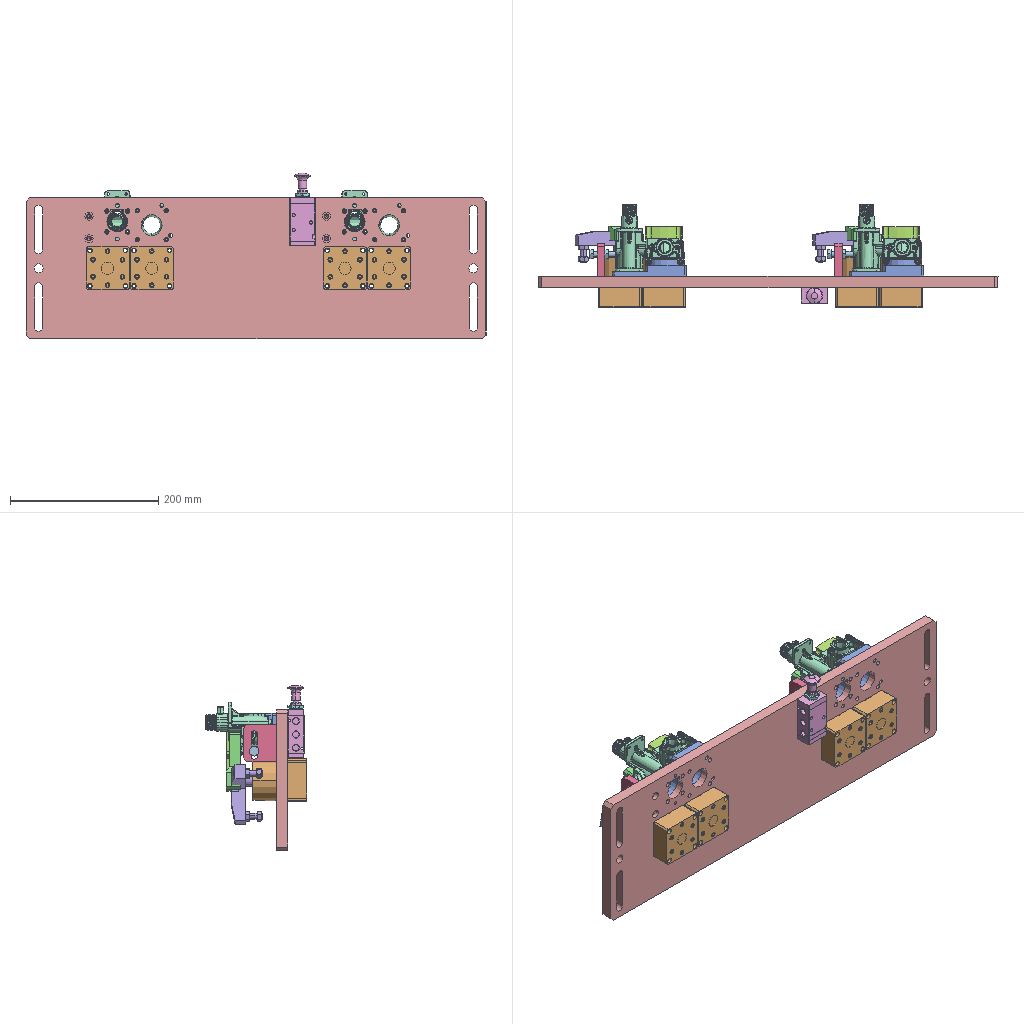Assembly | SolidWorks | 26 different items | 41 placed | box 620 x 137 x 223 mm
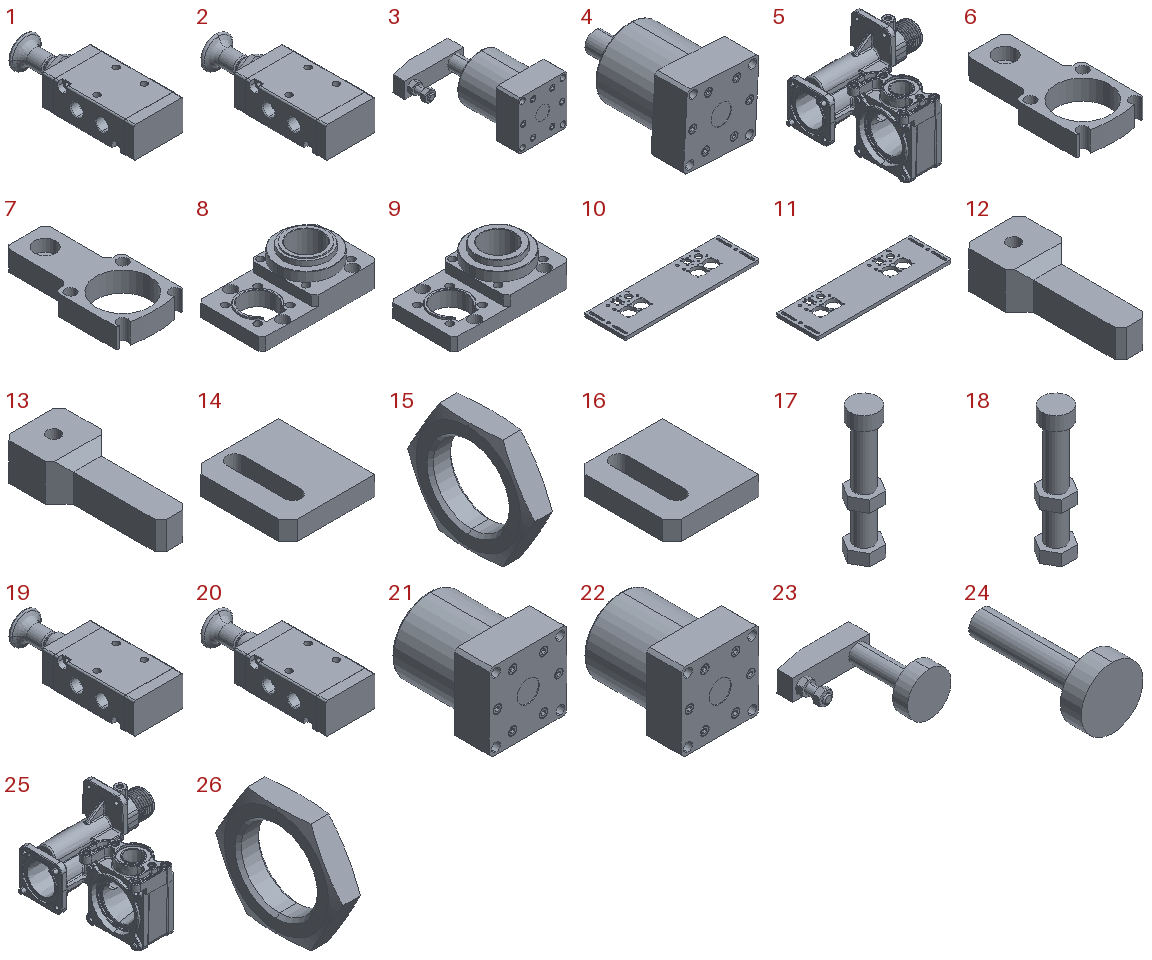Parts list (item | name | quantity | parent item | size | volume | features):
1 | (subassembly) | x1 | - | 35 x 98 x 22 mm | 51769 mm3 | -
2 | (subassembly) | x1 | - | 35 x 98 x 22 mm | 51769 mm3 | -
3 | (subassembly) | x4 | - | 88 x 124 x 58 mm | 194195 mm3 | -
4 | (subassembly) | x1 | - | 60.922 x 101.833 x 60.922 mm | 171940 mm3 | -
5 | - | x1 | - | - | - | features BaseBody 3, RefSurface 3
6 | - | x2 | - | 50 x 97 x 15 mm | 33774 mm3 | features ICE 4, Chamfer 1, Cut 1, Extrusion 1
7 | - | x1 | - | 50 x 97 x 15 mm | 33774 mm3 | features BaseBody 1
8 | - | x2 | - | 100 x 56 x 32.8 mm | 73783 mm3 | features ICE 6, Cut 3, Fillet 3, Chamfer 1, Extrusion 1, HoleWzd 1
9 | - | x1 | - | 100 x 56 x 32.8 mm | 75524 mm3 | features BaseBody 1
10 | - | x1 | - | 620 x 190 x 15 mm | 1473802 mm3 | features Cut 4, HoleWzd 4, ICE 2, LPattern 2, Chamfer 1, Extrusion 1, Fillet 1
11 | - | x1 | - | 620 x 190 x 15 mm | 1473802 mm3 | features BaseBody 1
12 | - | x2 | - | 30 x 77 x 20 mm | 24023 mm3 | features Chamfer 4, ICE 3, Cut 1, Extrusion 1
13 | - | x1 | - | 30 x 77 x 20 mm | 24023 mm3 | features BaseBody 1
14 | - | x2 | - | 45 x 50 x 10 mm | 18367 mm3 | features Chamfer 1, Extrusion 1, HoleWzd 1, ICE 1
15 | - | x1 | - | 4 x 21.554 x 18.667 mm | 652.633 mm3 | features BaseBody 1
16 | - | x1 | - | 45 x 50 x 10 mm | 18367 mm3 | features BaseBody 1
17 | - | x2 | - | 13.834 x 12.139 x 56 mm | 3933 mm3 | features ICE 2, Extrusion 1, LPattern 1
18 | - | x1 | - | 13.834 x 12.139 x 56 mm | 3933 mm3 | features BaseBody 1
19 | - | x1 | in 1 | 35 x 98 x 22 mm | 51117 mm3 | features BaseBody 1
20 | - | x1 | - | 35 x 98 x 22 mm | 51117 mm3 | features BaseBody 1
21 | - | x4 | in 3 | 58 x 74 x 58 mm | 141340 mm3 | features BaseBody 1
22 | - | x1 | - | 58 x 74 x 58 mm | 141332 mm3 | features BaseBody 1
23 | - | x4 | in 3 | 78.8 x 84 x 39.6 mm | 52858 mm3 | features BaseBody 1
24 | - | x1 | - | 39.6 x 84 x 39.6 mm | 30608 mm3 | features BaseBody 1
25 | - | x2 | - | - | - | features RefSurface 4, BaseBody 2
26 | - | x1 | in 1 | 4 x 21.554 x 18.667 mm | 652.692 mm3 | features BaseBody 1
Mates (type | each side: item.copy, entity, surface, feature):
In the top assembly
Parallel | 25.1 face plane Surface-input1 | 10.1 face plane Boss-Extrude1
Parallel | 25.1 face plane Surface-input1 | 8.1 face plane Boss-Extrude1
DistanceDim | 25.1 edge | 8.1 face plane Boss-Extrude1
Parallel | 10.1 face plane Boss-Extrude1 | 8.1 face plane Boss-Extrude1
DistanceDim | 10.1 face plane Boss-Extrude1 | 8.1 face plane Boss-Extrude1 | 2 times
Coincident | 25.1 face plane Surface-input1 | 8.1 face plane Boss-Extrude1
Coincident | 10.1 face plane Cut-Extrude3 | 8.1 face plane Boss-Extrude1
Coincident | 10.1 face plane Boss-Extrude1 | 19.1 face plane Input1 | 2 times
DistanceDim | 10.1 face plane Boss-Extrude1 | 19.1 face plane Input1
Coincident | 10.1 face plane Boss-Extrude1 | 21.1 face plane Input1
Concentric | 6.1 face cylinder Cut-Extrude3 | 23.1 face cylinder Input1
Coincident | 6.1 face plane Cut-Extrude3 | 23.1 face plane Input1
Parallel | 10.1 face plane Boss-Extrude1 | 21.1 face plane Input1
DistanceDim | 10.1 face plane Boss-Extrude1 | 21.1 face plane Input1
LimitPlanarAngleDim | 21.1 face plane Input1 | 6.1 face plane Boss-Extrude1
Coincident | 10.1 face plane Boss-Extrude1 | 21.2 face plane Input1
Concentric | 10.1 face cylinder Cut-Extrude6 | 21.2 face cylinder Input1
Concentric | 12.1 face cylinder Cut-Extrude2 | 23.2 face cylinder Input1
Coincident | 12.1 face plane Cut-Extrude1 | 23.2 face plane Input1
Parallel | 10.1 face plane Boss-Extrude1 | 21.2 face plane Input1
DistanceDim | 8.1 face plane Boss-Extrude1 | 21.1 face plane Input1
LimitPlanarAngleDim | 21.2 face plane Input1 | 12.1 face plane Cut-Extrude3
Coincident | 25.1 face plane Surface-input1 | 8.1 face plane Cut-Extrude2
Coincident | 10.1 face plane Boss-Extrude1 | 14.1 face plane Boss-Extrude1
DistanceDim | 8.1 face plane Boss-Extrude1 | 14.1 face plane Boss-Extrude1
DistanceDim | 10.1 face plane Boss-Extrude1 | 14.1 face plane Boss-Extrude1
Width | 14.1 face plane Cut-Extrude1 | 14.1 face plane Cut-Extrude1 | 17.1 face cylinder Boss-Extrude1
Parallel | 14.1 face plane Boss-Extrude1 | 17.1 face plane Boss-Extrude1
DistanceDim | 14.1 face plane Boss-Extrude1 | 17.1 face plane Boss-Extrude1
In subassembly 3
LimitDistanceDim | 21.3 face plane Input1 | 23.3 face plane Input1
Concentric | 21.3 face cylinder Input1 | 23.3 face cylinder Input1